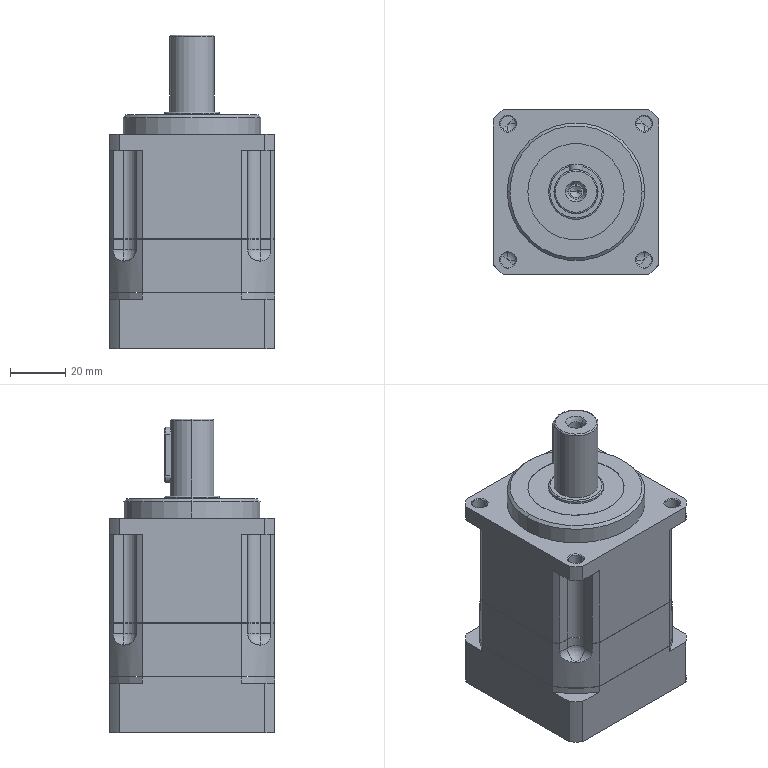Part | SolidWorks | features ICE 22, CirPattern 8, Fillet 5, Chamfer 3, 3DProfileFeature 2, HoleWzd 2, BlendCut 1, Extrusion 1 | 3 solids | 264 faces | box 60 x 60 x 114 mm | volume 258118 mm3 | plane 119 | cylinder 110 | cone 27 | torus 8 | commonest cylinder face diameters 70 x16 6 x12 8 x12 5.5 x10 50 x9 3.3 x8